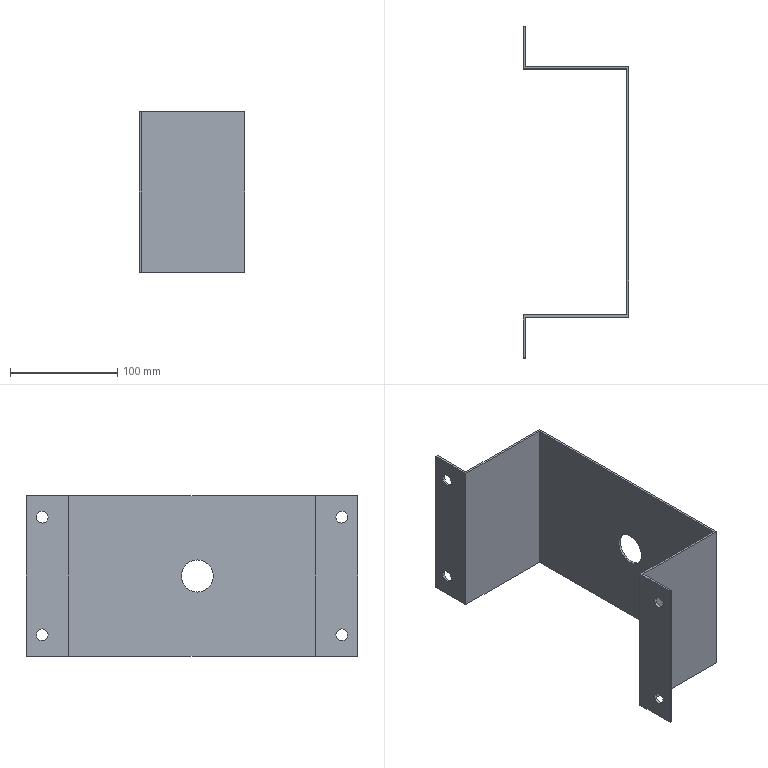Part | NX | features solid 2 | 1 solid | 19 faces | box 99 x 310 x 150 mm | volume 149026 mm3 | plane 14 | cylinder 5 | commonest cylinder face diameters 11 x4 30 x1
STEP:
#1=CARTESIAN_POINT('',(-1162.,-459.5,-415.));
#2=VERTEX_POINT('',#1);
#3=CARTESIAN_POINT('',(-1162.,-465.,-415.));
#4=DIRECTION('',(-1.,0.,0.));
#5=DIRECTION('',(0.,1.,0.));
#6=AXIS2_PLACEMENT_3D('',#3,#4,#5);
#7=CIRCLE('',#6,5.5);
#8=EDGE_CURVE('',#2,#2,#7,.T.);
#9=ORIENTED_EDGE('',*,*,#8,.F.);
#10=EDGE_LOOP('',(#9));
#11=FACE_BOUND('',#10,.T.);
#12=CARTESIAN_POINT('',(-1162.,-440.,-285.));
#13=VERTEX_POINT('',#12);
#14=CARTESIAN_POINT('',(-1162.,-440.,-435.));
#15=VERTEX_POINT('',#14);
#16=CARTESIAN_POINT('',(-1162.,-440.,-300.));
#17=DIRECTION('',(0.,0.,-1.));
#18=VECTOR('',#17,1000.);
#19=LINE('',#16,#18);
#20=EDGE_CURVE('',#13,#15,#19,.T.);
#21=ORIENTED_EDGE('',*,*,#20,.T.);
#22=CARTESIAN_POINT('',(-1162.,-480.,-435.));
#23=VERTEX_POINT('',#22);
#24=CARTESIAN_POINT('',(-1162.,-385.,-435.));
#25=DIRECTION('',(0.,1.,0.));
#26=VECTOR('',#25,1000.);
#27=LINE('',#24,#26);
#28=EDGE_CURVE('',#23,#15,#27,.T.);
#29=ORIENTED_EDGE('',*,*,#28,.F.);
#30=CARTESIAN_POINT('',(-1162.,-480.,-285.));
#31=VERTEX_POINT('',#30);
#32=CARTESIAN_POINT('',(-1162.,-480.,-300.));
#33=DIRECTION('',(0.,0.,-1.));
#34=VECTOR('',#33,1000.);
#35=LINE('',#32,#34);
#36=EDGE_CURVE('',#31,#23,#35,.T.);
#37=ORIENTED_EDGE('',*,*,#36,.F.);
#38=CARTESIAN_POINT('',(-1162.,-385.,-285.));
#39=DIRECTION('',(0.,1.,0.));
#40=VECTOR('',#39,1000.);
#41=LINE('',#38,#40);
#42=EDGE_CURVE('',#31,#13,#41,.T.);
#43=ORIENTED_EDGE('',*,*,#42,.T.);
#44=EDGE_LOOP('',(#21,#29,#37,#43));
#45=FACE_BOUND('',#44,.T.);
#46=CARTESIAN_POINT('',(-1162.,-459.5,-305.));
#47=VERTEX_POINT('',#46);
#48=CARTESIAN_POINT('',(-1162.,-465.,-305.));
#49=DIRECTION('',(1.,0.,0.));
#50=DIRECTION('',(0.,1.,0.));
#51=AXIS2_PLACEMENT_3D('',#48,#49,#50);
#52=CIRCLE('',#51,5.5);
#53=EDGE_CURVE('',#47,#47,#52,.T.);
#54=ORIENTED_EDGE('',*,*,#53,.T.);
#55=EDGE_LOOP('',(#54));
#56=FACE_BOUND('',#55,.T.);
#57=CARTESIAN_POINT('',(-1162.,-385.,-300.));
#58=DIRECTION('',(-1.,0.,0.));
#59=DIRECTION('',(0.,0.,1.));
#60=AXIS2_PLACEMENT_3D('',#57,#58,#59);
#61=PLANE('',#60);
#62=ADVANCED_FACE('',(#11,#45,#56),#61,.T.);
#63=CARTESIAN_POINT('',(-1160.,-465.,-409.5));
#64=VERTEX_POINT('',#63);
#65=CARTESIAN_POINT('',(-1160.,-465.,-415.));
#66=DIRECTION('',(-1.,0.,0.));
#67=DIRECTION('',(0.,0.,1.));
#68=AXIS2_PLACEMENT_3D('',#65,#66,#67);
#69=CIRCLE('',#68,5.5);
#70=EDGE_CURVE('',#64,#64,#69,.T.);
#71=ORIENTED_EDGE('',*,*,#70,.T.);
#72=EDGE_LOOP('',(#71));
#73=FACE_BOUND('',#72,.T.);
#74=CARTESIAN_POINT('',(-1160.,-442.,-435.));
#75=VERTEX_POINT('',#74);
#76=CARTESIAN_POINT('',(-1160.,-480.,-435.));
#77=VERTEX_POINT('',#76);
#78=CARTESIAN_POINT('',(-1160.,-385.,-435.));
#79=DIRECTION('',(0.,-1.,0.));
#80=VECTOR('',#79,1000.);
#81=LINE('',#78,#80);
#82=EDGE_CURVE('',#75,#77,#81,.T.);
#83=ORIENTED_EDGE('',*,*,#82,.F.);
#84=CARTESIAN_POINT('',(-1160.,-442.,-285.));
#85=VERTEX_POINT('',#84);
#86=CARTESIAN_POINT('',(-1160.,-442.,-300.));
#87=DIRECTION('',(0.,0.,-1.));
#88=VECTOR('',#87,1000.);
#89=LINE('',#86,#88);
#90=EDGE_CURVE('',#85,#75,#89,.T.);
#91=ORIENTED_EDGE('',*,*,#90,.F.);
#92=CARTESIAN_POINT('',(-1160.,-480.,-285.));
#93=VERTEX_POINT('',#92);
#94=CARTESIAN_POINT('',(-1160.,-385.,-285.));
#95=DIRECTION('',(0.,-1.,0.));
#96=VECTOR('',#95,1000.);
#97=LINE('',#94,#96);
#98=EDGE_CURVE('',#85,#93,#97,.T.);
#99=ORIENTED_EDGE('',*,*,#98,.T.);
#100=CARTESIAN_POINT('',(-1160.,-480.,-300.));
#101=DIRECTION('',(0.,0.,-1.));
#102=VECTOR('',#101,1000.);
#103=LINE('',#100,#102);
#104=EDGE_CURVE('',#93,#77,#103,.T.);
#105=ORIENTED_EDGE('',*,*,#104,.T.);
#106=EDGE_LOOP('',(#83,#91,#99,#105));
#107=FACE_BOUND('',#106,.T.);
#108=CARTESIAN_POINT('',(-1160.,-465.,-299.5));
#109=VERTEX_POINT('',#108);
#110=CARTESIAN_POINT('',(-1160.,-465.,-305.));
#111=DIRECTION('',(-1.,0.,0.));
#112=DIRECTION('',(0.,0.,1.));
#113=AXIS2_PLACEMENT_3D('',#110,#111,#112);
#114=CIRCLE('',#113,5.5);
#115=EDGE_CURVE('',#109,#109,#114,.F.);
#116=ORIENTED_EDGE('',*,*,#115,.F.);
#117=EDGE_LOOP('',(#116));
#118=FACE_BOUND('',#117,.T.);
#119=CARTESIAN_POINT('',(-1160.,-385.,-300.));
#120=DIRECTION('',(-1.,0.,0.));
#121=DIRECTION('',(0.,0.,-1.));
#122=AXIS2_PLACEMENT_3D('',#119,#120,#121);
#123=PLANE('',#122);
#124=ADVANCED_FACE('',(#73,#107,#118),#123,.F.);
#125=CARTESIAN_POINT('',(-1162.,-210.,-285.));
#126=VERTEX_POINT('',#125);
#127=CARTESIAN_POINT('',(-1162.,-210.,-435.));
#128=VERTEX_POINT('',#127);
#129=CARTESIAN_POINT('',(-1162.,-210.,-300.));
#130=DIRECTION('',(0.,0.,-1.));
#131=VECTOR('',#130,1000.);
#132=LINE('',#129,#131);
#133=EDGE_CURVE('',#126,#128,#132,.T.);
#134=ORIENTED_EDGE('',*,*,#133,.F.);
#135=CARTESIAN_POINT('',(-1162.,-170.,-285.));
#136=VERTEX_POINT('',#135);
#137=CARTESIAN_POINT('',(-1162.,-265.,-285.));
#138=DIRECTION('',(0.,-1.,0.));
#139=VECTOR('',#138,1000.);
#140=LINE('',#137,#139);
#141=EDGE_CURVE('',#136,#126,#140,.T.);
#142=ORIENTED_EDGE('',*,*,#141,.F.);
#143=CARTESIAN_POINT('',(-1162.,-170.,-435.));
#144=VERTEX_POINT('',#143);
#145=CARTESIAN_POINT('',(-1162.,-170.,-300.));
#146=DIRECTION('',(0.,0.,-1.));
#147=VECTOR('',#146,1000.);
#148=LINE('',#145,#147);
#149=EDGE_CURVE('',#136,#144,#148,.T.);
#150=ORIENTED_EDGE('',*,*,#149,.T.);
#151=CARTESIAN_POINT('',(-1162.,-265.,-435.));
#152=DIRECTION('',(0.,-1.,0.));
#153=VECTOR('',#152,1000.);
#154=LINE('',#151,#153);
#155=EDGE_CURVE('',#144,#128,#154,.T.);
#156=ORIENTED_EDGE('',*,*,#155,.T.);
#157=EDGE_LOOP('',(#134,#142,#150,#156));
#158=FACE_BOUND('',#157,.T.);
#159=CARTESIAN_POINT('',(-1162.,-190.5,-305.));
#160=VERTEX_POINT('',#159);
#161=CARTESIAN_POINT('',(-1162.,-185.,-305.));
#162=DIRECTION('',(-1.,0.,0.));
#163=DIRECTION('',(0.,-1.,0.));
#164=AXIS2_PLACEMENT_3D('',#161,#162,#163);
#165=CIRCLE('',#164,5.5);
#166=EDGE_CURVE('',#160,#160,#165,.T.);
#167=ORIENTED_EDGE('',*,*,#166,.F.);
#168=EDGE_LOOP('',(#167));
#169=FACE_BOUND('',#168,.T.);
#170=CARTESIAN_POINT('',(-1162.,-190.5,-415.));
#171=VERTEX_POINT('',#170);
#172=CARTESIAN_POINT('',(-1162.,-185.,-415.));
#173=DIRECTION('',(1.,0.,0.));
#174=DIRECTION('',(0.,-1.,0.));
#175=AXIS2_PLACEMENT_3D('',#172,#173,#174);
#176=CIRCLE('',#175,5.5);
#177=EDGE_CURVE('',#171,#171,#176,.T.);
#178=ORIENTED_EDGE('',*,*,#177,.T.);
#179=EDGE_LOOP('',(#178));
#180=FACE_BOUND('',#179,.T.);
#181=CARTESIAN_POINT('',(-1162.,-265.,-300.));
#182=DIRECTION('',(-1.,0.,0.));
#183=DIRECTION('',(0.,0.,1.));
#184=AXIS2_PLACEMENT_3D('',#181,#182,#183);
#185=PLANE('',#184);
#186=ADVANCED_FACE('',(#158,#169,#180),#185,.T.);
#187=CARTESIAN_POINT('',(-1160.,-208.,-435.));
#188=VERTEX_POINT('',#187);
#189=CARTESIAN_POINT('',(-1160.,-170.,-435.));
#190=VERTEX_POINT('',#189);
#191=CARTESIAN_POINT('',(-1160.,-385.,-435.));
#192=DIRECTION('',(0.,1.,0.));
#193=VECTOR('',#192,1000.);
#194=LINE('',#191,#193);
#195=EDGE_CURVE('',#188,#190,#194,.T.);
#196=ORIENTED_EDGE('',*,*,#195,.T.);
#197=CARTESIAN_POINT('',(-1160.,-170.,-285.));
#198=VERTEX_POINT('',#197);
#199=CARTESIAN_POINT('',(-1160.,-170.,-300.));
#200=DIRECTION('',(0.,0.,-1.));
#201=VECTOR('',#200,1000.);
#202=LINE('',#199,#201);
#203=EDGE_CURVE('',#198,#190,#202,.T.);
#204=ORIENTED_EDGE('',*,*,#203,.F.);
#205=CARTESIAN_POINT('',(-1160.,-208.,-285.));
#206=VERTEX_POINT('',#205);
#207=CARTESIAN_POINT('',(-1160.,-385.,-285.));
#208=DIRECTION('',(0.,1.,0.));
#209=VECTOR('',#208,1000.);
#210=LINE('',#207,#209);
#211=EDGE_CURVE('',#206,#198,#210,.T.);
#212=ORIENTED_EDGE('',*,*,#211,.F.);
#213=CARTESIAN_POINT('',(-1160.,-208.,-300.));
#214=DIRECTION('',(0.,0.,-1.));
#215=VECTOR('',#214,1000.);
#216=LINE('',#213,#215);
#217=EDGE_CURVE('',#206,#188,#216,.T.);
#218=ORIENTED_EDGE('',*,*,#217,.T.);
#219=EDGE_LOOP('',(#196,#204,#212,#218));
#220=FACE_BOUND('',#219,.T.);
#221=CARTESIAN_POINT('',(-1160.,-185.,-299.5));
#222=VERTEX_POINT('',#221);
#223=CARTESIAN_POINT('',(-1160.,-185.,-305.));
#224=DIRECTION('',(-1.,0.,0.));
#225=DIRECTION('',(0.,0.,1.));
#226=AXIS2_PLACEMENT_3D('',#223,#224,#225);
#227=CIRCLE('',#226,5.5);
#228=EDGE_CURVE('',#222,#222,#227,.T.);
#229=ORIENTED_EDGE('',*,*,#228,.T.);
#230=EDGE_LOOP('',(#229));
#231=FACE_BOUND('',#230,.T.);
#232=CARTESIAN_POINT('',(-1160.,-185.,-409.5));
#233=VERTEX_POINT('',#232);
#234=CARTESIAN_POINT('',(-1160.,-185.,-415.));
#235=DIRECTION('',(-1.,0.,0.));
#236=DIRECTION('',(0.,0.,1.));
#237=AXIS2_PLACEMENT_3D('',#234,#235,#236);
#238=CIRCLE('',#237,5.5);
#239=EDGE_CURVE('',#233,#233,#238,.F.);
#240=ORIENTED_EDGE('',*,*,#239,.F.);
#241=EDGE_LOOP('',(#240));
#242=FACE_BOUND('',#241,.T.);
#243=CARTESIAN_POINT('',(-1160.,-265.,-300.));
#244=DIRECTION('',(-1.,0.,0.));
#245=DIRECTION('',(0.,0.,-1.));
#246=AXIS2_PLACEMENT_3D('',#243,#244,#245);
#247=PLANE('',#246);
#248=ADVANCED_FACE('',(#220,#231,#242),#247,.F.);
#249=ORIENTED_EDGE('',*,*,#90,.T.);
#250=CARTESIAN_POINT('',(-1063.,-442.,-435.));
#251=VERTEX_POINT('',#250);
#252=CARTESIAN_POINT('',(-1160.,-442.,-435.));
#253=DIRECTION('',(1.,0.,0.));
#254=VECTOR('',#253,1000.);
#255=LINE('',#252,#254);
#256=EDGE_CURVE('',#75,#251,#255,.T.);
#257=ORIENTED_EDGE('',*,*,#256,.T.);
#258=CARTESIAN_POINT('',(-1063.,-442.,-285.));
#259=VERTEX_POINT('',#258);
#260=CARTESIAN_POINT('',(-1063.,-442.,-300.));
#261=DIRECTION('',(0.,0.,-1.));
#262=VECTOR('',#261,1000.);
#263=LINE('',#260,#262);
#264=EDGE_CURVE('',#259,#251,#263,.T.);
#265=ORIENTED_EDGE('',*,*,#264,.F.);
#266=CARTESIAN_POINT('',(-1160.,-442.,-285.));
#267=DIRECTION('',(1.,0.,0.));
#268=VECTOR('',#267,1000.);
#269=LINE('',#266,#268);
#270=EDGE_CURVE('',#85,#259,#269,.T.);
#271=ORIENTED_EDGE('',*,*,#270,.F.);
#272=EDGE_LOOP('',(#249,#257,#265,#271));
#273=FACE_BOUND('',#272,.T.);
#274=CARTESIAN_POINT('',(-1160.,-442.,-300.));
#275=DIRECTION('',(0.,1.,0.));
#276=DIRECTION('',(0.,0.,-1.));
#277=AXIS2_PLACEMENT_3D('',#274,#275,#276);
#278=PLANE('',#277);
#279=ADVANCED_FACE('',(#273),#278,.F.);
#280=CARTESIAN_POINT('',(-1063.,-208.,-285.));
#281=VERTEX_POINT('',#280);
#282=CARTESIAN_POINT('',(-1063.,-385.,-285.));
#283=DIRECTION('',(0.,1.,0.));
#284=VECTOR('',#283,1000.);
#285=LINE('',#282,#284);
#286=EDGE_CURVE('',#259,#281,#285,.T.);
#287=ORIENTED_EDGE('',*,*,#286,.T.);
#288=CARTESIAN_POINT('',(-1160.,-208.,-285.));
#289=DIRECTION('',(1.,0.,0.));
#290=VECTOR('',#289,1000.);
#291=LINE('',#288,#290);
#292=EDGE_CURVE('',#206,#281,#291,.T.);
#293=ORIENTED_EDGE('',*,*,#292,.F.);
#294=ORIENTED_EDGE('',*,*,#211,.T.);
#295=CARTESIAN_POINT('',(-1160.,-170.,-285.));
#296=DIRECTION('',(1.,0.,0.));
#297=VECTOR('',#296,1000.);
#298=LINE('',#295,#297);
#299=EDGE_CURVE('',#136,#198,#298,.T.);
#300=ORIENTED_EDGE('',*,*,#299,.F.);
#301=ORIENTED_EDGE('',*,*,#141,.T.);
#302=CARTESIAN_POINT('',(-1065.,-210.,-285.));
#303=VERTEX_POINT('',#302);
#304=CARTESIAN_POINT('',(-1160.,-210.,-285.));
#305=DIRECTION('',(1.,0.,0.));
#306=VECTOR('',#305,1000.);
#307=LINE('',#304,#306);
#308=EDGE_CURVE('',#126,#303,#307,.T.);
#309=ORIENTED_EDGE('',*,*,#308,.T.);
#310=CARTESIAN_POINT('',(-1065.,-440.,-285.));
#311=VERTEX_POINT('',#310);
#312=CARTESIAN_POINT('',(-1065.,-385.,-285.));
#313=DIRECTION('',(0.,1.,0.));
#314=VECTOR('',#313,1000.);
#315=LINE('',#312,#314);
#316=EDGE_CURVE('',#311,#303,#315,.T.);
#317=ORIENTED_EDGE('',*,*,#316,.F.);
#318=CARTESIAN_POINT('',(-1160.,-440.,-285.));
#319=DIRECTION('',(1.,0.,0.));
#320=VECTOR('',#319,1000.);
#321=LINE('',#318,#320);
#322=EDGE_CURVE('',#13,#311,#321,.T.);
#323=ORIENTED_EDGE('',*,*,#322,.F.);
#324=ORIENTED_EDGE('',*,*,#42,.F.);
#325=CARTESIAN_POINT('',(-1160.,-480.,-285.));
#326=DIRECTION('',(1.,0.,0.));
#327=VECTOR('',#326,1000.);
#328=LINE('',#325,#327);
#329=EDGE_CURVE('',#31,#93,#328,.T.);
#330=ORIENTED_EDGE('',*,*,#329,.T.);
#331=ORIENTED_EDGE('',*,*,#98,.F.);
#332=ORIENTED_EDGE('',*,*,#270,.T.);
#333=EDGE_LOOP('',(#287,#293,#294,#300,#301,#309,#317,#323,#324,#330,#331,#332));
#334=FACE_BOUND('',#333,.T.);
#335=CARTESIAN_POINT('',(-1160.,-385.,-285.));
#336=DIRECTION('',(0.,0.,-1.));
#337=DIRECTION('',(-1.,0.,0.));
#338=AXIS2_PLACEMENT_3D('',#335,#336,#337);
#339=PLANE('',#338);
#340=ADVANCED_FACE('',(#334),#339,.F.);
#341=CARTESIAN_POINT('',(-1065.,-440.,-435.));
#342=VERTEX_POINT('',#341);
#343=CARTESIAN_POINT('',(-1065.,-210.,-435.));
#344=VERTEX_POINT('',#343);
#345=CARTESIAN_POINT('',(-1065.,-385.,-435.));
#346=DIRECTION('',(0.,1.,0.));
#347=VECTOR('',#346,1000.);
#348=LINE('',#345,#347);
#349=EDGE_CURVE('',#342,#344,#348,.T.);
#350=ORIENTED_EDGE('',*,*,#349,.T.);
#351=CARTESIAN_POINT('',(-1160.,-210.,-435.));
#352=DIRECTION('',(1.,0.,0.));
#353=VECTOR('',#352,1000.);
#354=LINE('',#351,#353);
#355=EDGE_CURVE('',#128,#344,#354,.T.);
#356=ORIENTED_EDGE('',*,*,#355,.F.);
#357=ORIENTED_EDGE('',*,*,#155,.F.);
#358=CARTESIAN_POINT('',(-1160.,-170.,-435.));
#359=DIRECTION('',(1.,0.,0.));
#360=VECTOR('',#359,1000.);
#361=LINE('',#358,#360);
#362=EDGE_CURVE('',#144,#190,#361,.T.);
#363=ORIENTED_EDGE('',*,*,#362,.T.);
#364=ORIENTED_EDGE('',*,*,#195,.F.);
#365=CARTESIAN_POINT('',(-1063.,-208.,-435.));
#366=VERTEX_POINT('',#365);
#367=CARTESIAN_POINT('',(-1160.,-208.,-435.));
#368=DIRECTION('',(1.,0.,0.));
#369=VECTOR('',#368,1000.);
#370=LINE('',#367,#369);
#371=EDGE_CURVE('',#188,#366,#370,.T.);
#372=ORIENTED_EDGE('',*,*,#371,.T.);
#373=CARTESIAN_POINT('',(-1063.,-385.,-435.));
#374=DIRECTION('',(0.,1.,0.));
#375=VECTOR('',#374,1000.);
#376=LINE('',#373,#375);
#377=EDGE_CURVE('',#251,#366,#376,.T.);
#378=ORIENTED_EDGE('',*,*,#377,.F.);
#379=ORIENTED_EDGE('',*,*,#256,.F.);
#380=ORIENTED_EDGE('',*,*,#82,.T.);
#381=CARTESIAN_POINT('',(-1160.,-480.,-435.));
#382=DIRECTION('',(1.,0.,0.));
#383=VECTOR('',#382,1000.);
#384=LINE('',#381,#383);
#385=EDGE_CURVE('',#23,#77,#384,.T.);
#386=ORIENTED_EDGE('',*,*,#385,.F.);
#387=ORIENTED_EDGE('',*,*,#28,.T.);
#388=CARTESIAN_POINT('',(-1160.,-440.,-435.));
#389=DIRECTION('',(1.,0.,0.));
#390=VECTOR('',#389,1000.);
#391=LINE('',#388,#390);
#392=EDGE_CURVE('',#15,#342,#391,.T.);
#393=ORIENTED_EDGE('',*,*,#392,.T.);
#394=EDGE_LOOP('',(#350,#356,#357,#363,#364,#372,#378,#379,#380,#386,#387,#393));
#395=FACE_BOUND('',#394,.T.);
#396=CARTESIAN_POINT('',(-1160.,-385.,-435.));
#397=DIRECTION('',(0.,0.,-1.));
#398=DIRECTION('',(-1.,0.,0.));
#399=AXIS2_PLACEMENT_3D('',#396,#397,#398);
#400=PLANE('',#399);
#401=ADVANCED_FACE('',(#395),#400,.T.);
#402=CARTESIAN_POINT('',(-1065.,-440.,-300.));
#403=DIRECTION('',(0.,0.,-1.));
#404=VECTOR('',#403,1000.);
#405=LINE('',#402,#404);
#406=EDGE_CURVE('',#311,#342,#405,.T.);
#407=ORIENTED_EDGE('',*,*,#406,.T.);
#408=ORIENTED_EDGE('',*,*,#392,.F.);
#409=ORIENTED_EDGE('',*,*,#20,.F.);
#410=ORIENTED_EDGE('',*,*,#322,.T.);
#411=EDGE_LOOP('',(#407,#408,#409,#410));
#412=FACE_BOUND('',#411,.T.);
#413=CARTESIAN_POINT('',(-1160.,-440.,-300.));
#414=DIRECTION('',(0.,1.,0.));
#415=DIRECTION('',(0.,0.,-1.));
#416=AXIS2_PLACEMENT_3D('',#413,#414,#415);
#417=PLANE('',#416);
#418=ADVANCED_FACE('',(#412),#417,.T.);
#419=ORIENTED_EDGE('',*,*,#104,.F.);
#420=ORIENTED_EDGE('',*,*,#329,.F.);
#421=ORIENTED_EDGE('',*,*,#36,.T.);
#422=ORIENTED_EDGE('',*,*,#385,.T.);
#423=EDGE_LOOP('',(#419,#420,#421,#422));
#424=FACE_BOUND('',#423,.T.);
#425=CARTESIAN_POINT('',(-1160.,-480.,-300.));
#426=DIRECTION('',(0.,1.,0.));
#427=DIRECTION('',(0.,0.,-1.));
#428=AXIS2_PLACEMENT_3D('',#425,#426,#427);
#429=PLANE('',#428);
#430=ADVANCED_FACE('',(#424),#429,.F.);
#431=CARTESIAN_POINT('',(-1065.,-330.,-345.));
#432=VERTEX_POINT('',#431);
#433=CARTESIAN_POINT('',(-1065.,-330.,-360.));
#434=DIRECTION('',(-1.,0.,0.));
#435=DIRECTION('',(0.,0.,1.));
#436=AXIS2_PLACEMENT_3D('',#433,#434,#435);
#437=CIRCLE('',#436,15.);
#438=EDGE_CURVE('',#432,#432,#437,.T.);
#439=ORIENTED_EDGE('',*,*,#438,.F.);
#440=EDGE_LOOP('',(#439));
#441=FACE_BOUND('',#440,.T.);
#442=ORIENTED_EDGE('',*,*,#316,.T.);
#443=CARTESIAN_POINT('',(-1065.,-210.,-300.));
#444=DIRECTION('',(0.,0.,-1.));
#445=VECTOR('',#444,1000.);
#446=LINE('',#443,#445);
#447=EDGE_CURVE('',#303,#344,#446,.T.);
#448=ORIENTED_EDGE('',*,*,#447,.T.);
#449=ORIENTED_EDGE('',*,*,#349,.F.);
#450=ORIENTED_EDGE('',*,*,#406,.F.);
#451=EDGE_LOOP('',(#442,#448,#449,#450));
#452=FACE_BOUND('',#451,.T.);
#453=CARTESIAN_POINT('',(-1065.,-385.,-300.));
#454=DIRECTION('',(-1.,0.,0.));
#455=DIRECTION('',(0.,0.,1.));
#456=AXIS2_PLACEMENT_3D('',#453,#454,#455);
#457=PLANE('',#456);
#458=ADVANCED_FACE('',(#441,#452),#457,.T.);
#459=CARTESIAN_POINT('',(-1063.,-330.,-345.));
#460=VERTEX_POINT('',#459);
#461=CARTESIAN_POINT('',(-1063.,-330.,-360.));
#462=DIRECTION('',(-1.,0.,0.));
#463=DIRECTION('',(0.,0.,1.));
#464=AXIS2_PLACEMENT_3D('',#461,#462,#463);
#465=CIRCLE('',#464,15.);
#466=EDGE_CURVE('',#460,#460,#465,.T.);
#467=ORIENTED_EDGE('',*,*,#466,.T.);
#468=EDGE_LOOP('',(#467));
#469=FACE_BOUND('',#468,.T.);
#470=ORIENTED_EDGE('',*,*,#377,.T.);
#471=CARTESIAN_POINT('',(-1063.,-208.,-300.));
#472=DIRECTION('',(0.,0.,-1.));
#473=VECTOR('',#472,1000.);
#474=LINE('',#471,#473);
#475=EDGE_CURVE('',#281,#366,#474,.T.);
#476=ORIENTED_EDGE('',*,*,#475,.F.);
#477=ORIENTED_EDGE('',*,*,#286,.F.);
#478=ORIENTED_EDGE('',*,*,#264,.T.);
#479=EDGE_LOOP('',(#470,#476,#477,#478));
#480=FACE_BOUND('',#479,.T.);
#481=CARTESIAN_POINT('',(-1063.,-385.,-300.));
#482=DIRECTION('',(-1.,0.,0.));
#483=DIRECTION('',(0.,0.,1.));
#484=AXIS2_PLACEMENT_3D('',#481,#482,#483);
#485=PLANE('',#484);
#486=ADVANCED_FACE('',(#469,#480),#485,.F.);
#487=ORIENTED_EDGE('',*,*,#217,.F.);
#488=ORIENTED_EDGE('',*,*,#292,.T.);
#489=ORIENTED_EDGE('',*,*,#475,.T.);
#490=ORIENTED_EDGE('',*,*,#371,.F.);
#491=EDGE_LOOP('',(#487,#488,#489,#490));
#492=FACE_BOUND('',#491,.T.);
#493=CARTESIAN_POINT('',(-1160.,-208.,-300.));
#494=DIRECTION('',(0.,-1.,0.));
#495=DIRECTION('',(0.,0.,-1.));
#496=AXIS2_PLACEMENT_3D('',#493,#494,#495);
#497=PLANE('',#496);
#498=ADVANCED_FACE('',(#492),#497,.F.);
#499=ORIENTED_EDGE('',*,*,#447,.F.);
#500=ORIENTED_EDGE('',*,*,#308,.F.);
#501=ORIENTED_EDGE('',*,*,#133,.T.);
#502=ORIENTED_EDGE('',*,*,#355,.T.);
#503=EDGE_LOOP('',(#499,#500,#501,#502));
#504=FACE_BOUND('',#503,.T.);
#505=CARTESIAN_POINT('',(-1160.,-210.,-300.));
#506=DIRECTION('',(0.,-1.,0.));
#507=DIRECTION('',(0.,0.,-1.));
#508=AXIS2_PLACEMENT_3D('',#505,#506,#507);
#509=PLANE('',#508);
#510=ADVANCED_FACE('',(#504),#509,.T.);
#511=ORIENTED_EDGE('',*,*,#203,.T.);
#512=ORIENTED_EDGE('',*,*,#362,.F.);
#513=ORIENTED_EDGE('',*,*,#149,.F.);
#514=ORIENTED_EDGE('',*,*,#299,.T.);
#515=EDGE_LOOP('',(#511,#512,#513,#514));
#516=FACE_BOUND('',#515,.T.);
#517=CARTESIAN_POINT('',(-1160.,-170.,-300.));
#518=DIRECTION('',(0.,-1.,0.));
#519=DIRECTION('',(0.,0.,-1.));
#520=AXIS2_PLACEMENT_3D('',#517,#518,#519);
#521=PLANE('',#520);
#522=ADVANCED_FACE('',(#516),#521,.F.);
#523=ORIENTED_EDGE('',*,*,#438,.T.);
#524=EDGE_LOOP('',(#523));
#525=FACE_BOUND('',#524,.T.);
#526=ORIENTED_EDGE('',*,*,#466,.F.);
#527=EDGE_LOOP('',(#526));
#528=FACE_BOUND('',#527,.T.);
#529=CARTESIAN_POINT('',(-1070.,-330.,-360.));
#530=DIRECTION('',(-1.,0.,0.));
#531=DIRECTION('',(0.,0.,1.));
#532=AXIS2_PLACEMENT_3D('',#529,#530,#531);
#533=CYLINDRICAL_SURFACE('',#532,15.);
#534=ADVANCED_FACE('',(#525,#528),#533,.F.);
#535=ORIENTED_EDGE('',*,*,#166,.T.);
#536=EDGE_LOOP('',(#535));
#537=FACE_BOUND('',#536,.T.);
#538=ORIENTED_EDGE('',*,*,#228,.F.);
#539=EDGE_LOOP('',(#538));
#540=FACE_BOUND('',#539,.T.);
#541=CARTESIAN_POINT('',(-1132.,-185.,-305.));
#542=DIRECTION('',(-1.,0.,0.));
#543=DIRECTION('',(0.,0.,1.));
#544=AXIS2_PLACEMENT_3D('',#541,#542,#543);
#545=CYLINDRICAL_SURFACE('',#544,5.5);
#546=ADVANCED_FACE('',(#537,#540),#545,.F.);
#547=ORIENTED_EDGE('',*,*,#177,.F.);
#548=EDGE_LOOP('',(#547));
#549=FACE_BOUND('',#548,.T.);
#550=ORIENTED_EDGE('',*,*,#239,.T.);
#551=EDGE_LOOP('',(#550));
#552=FACE_BOUND('',#551,.T.);
#553=CARTESIAN_POINT('',(-1132.,-185.,-415.));
#554=DIRECTION('',(-1.,0.,0.));
#555=DIRECTION('',(0.,0.,1.));
#556=AXIS2_PLACEMENT_3D('',#553,#554,#555);
#557=CYLINDRICAL_SURFACE('',#556,5.5);
#558=ADVANCED_FACE('',(#549,#552),#557,.F.);
#559=ORIENTED_EDGE('',*,*,#53,.F.);
#560=EDGE_LOOP('',(#559));
#561=FACE_BOUND('',#560,.T.);
#562=ORIENTED_EDGE('',*,*,#115,.T.);
#563=EDGE_LOOP('',(#562));
#564=FACE_BOUND('',#563,.T.);
#565=CARTESIAN_POINT('',(-1132.,-465.,-305.));
#566=DIRECTION('',(-1.,0.,0.));
#567=DIRECTION('',(0.,0.,1.));
#568=AXIS2_PLACEMENT_3D('',#565,#566,#567);
#569=CYLINDRICAL_SURFACE('',#568,5.5);
#570=ADVANCED_FACE('',(#561,#564),#569,.F.);
#571=ORIENTED_EDGE('',*,*,#8,.T.);
#572=EDGE_LOOP('',(#571));
#573=FACE_BOUND('',#572,.T.);
#574=ORIENTED_EDGE('',*,*,#70,.F.);
#575=EDGE_LOOP('',(#574));
#576=FACE_BOUND('',#575,.T.);
#577=CARTESIAN_POINT('',(-1132.,-465.,-415.));
#578=DIRECTION('',(-1.,0.,0.));
#579=DIRECTION('',(0.,0.,1.));
#580=AXIS2_PLACEMENT_3D('',#577,#578,#579);
#581=CYLINDRICAL_SURFACE('',#580,5.5);
#582=ADVANCED_FACE('',(#573,#576),#581,.F.);
#583=CLOSED_SHELL('',(#62,#124,#186,#248,#279,#340,#401,#418,#430,#458,#486,#498,#510,#522,#534,#546,#558,#570,#582));
#584=MANIFOLD_SOLID_BREP('',#583);
#585=(LENGTH_UNIT()NAMED_UNIT(*)SI_UNIT(.MILLI.,.METRE.));
#586=UNCERTAINTY_MEASURE_WITH_UNIT(LENGTH_MEASURE(0.00001),#585,'','');
#587=(NAMED_UNIT(*)PLANE_ANGLE_UNIT()SI_UNIT($,.RADIAN.));
#588=(NAMED_UNIT(*)SI_UNIT($,.STERADIAN.)SOLID_ANGLE_UNIT());
#589=(GEOMETRIC_REPRESENTATION_CONTEXT(3)GLOBAL_UNCERTAINTY_ASSIGNED_CONTEXT((#586))GLOBAL_UNIT_ASSIGNED_CONTEXT((#585,#587,#588))REPRESENTATION_CONTEXT('',''));
#590=ADVANCED_BREP_SHAPE_REPRESENTATION('',(#584),#589);